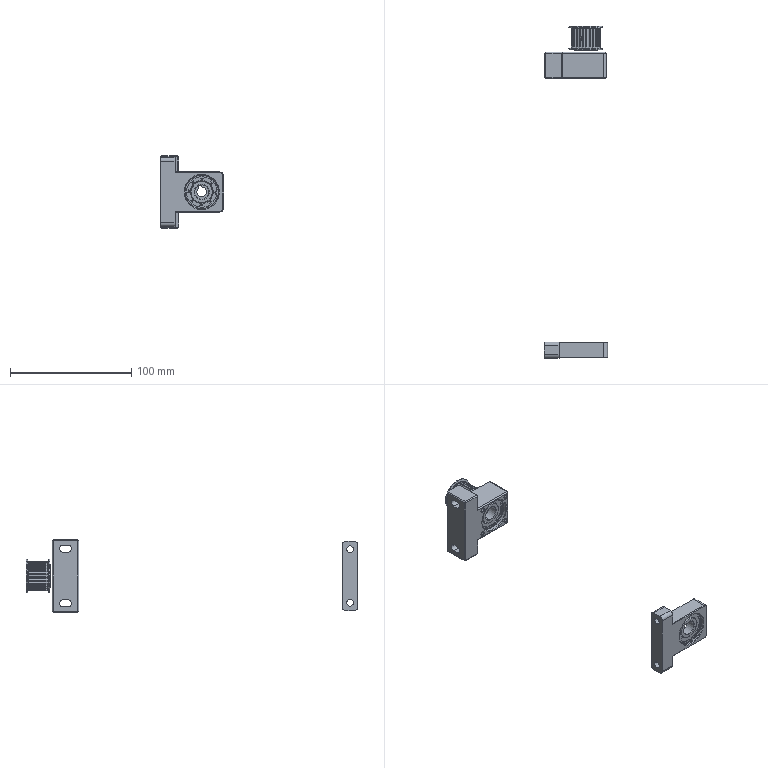Part | NX | features BREP 6 | 8 solids | 848 faces | box 52 x 273.5 x 60 mm | volume 59712 mm3 | cylinder 280 | plane 222 | sphere 192 | torus 96 | cone 58 | commonest cylinder face diameters 0.34 x69 2.06 x40 24.07 x26 25.2 x24 28 x14 17.4 x12